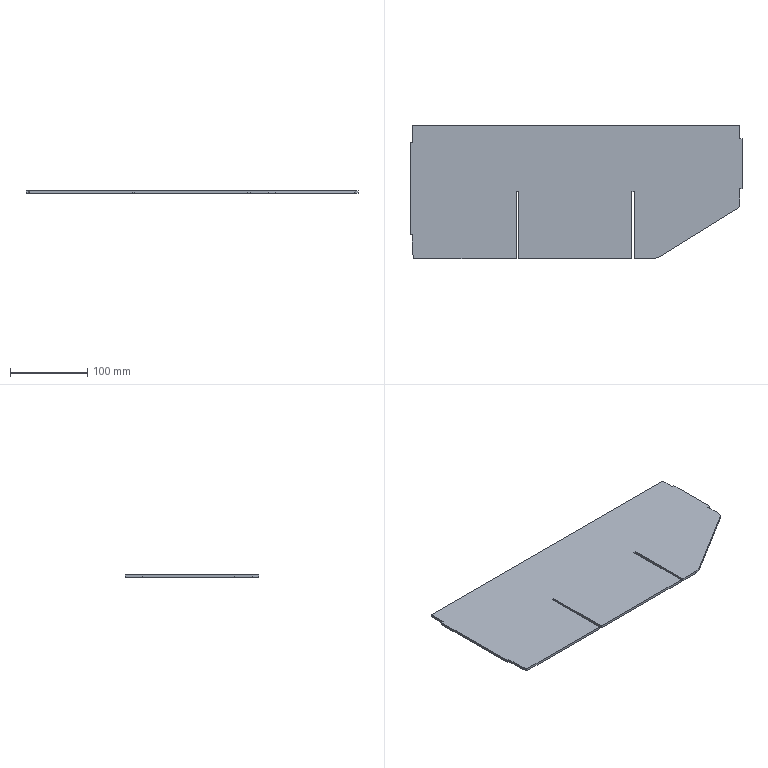Part | SolidWorks | features FlatPattern 1, SMBaseFlange 1, SheetMetal 1 | 1 solid | 26 faces | box 431 x 173.7 x 3.2 mm | volume 224566 mm3 | plane 26
STEP:
#1=CARTESIAN_POINT('',(206.522,-13.627,0.));
#2=VERTEX_POINT('',#1);
#3=CARTESIAN_POINT('',(-218.478,-13.627,0.));
#4=VERTEX_POINT('',#3);
#5=CARTESIAN_POINT('',(-218.478,-13.627,0.));
#6=DIRECTION('',(-1.,0.,0.));
#7=VECTOR('',#6,1000.);
#8=LINE('',#5,#7);
#9=EDGE_CURVE('',#2,#4,#8,.T.);
#10=ORIENTED_EDGE('',*,*,#9,.T.);
#11=CARTESIAN_POINT('',(-218.478,-13.627,3.2));
#12=VERTEX_POINT('',#11);
#13=CARTESIAN_POINT('',(-218.478,-13.627,3.2));
#14=DIRECTION('',(0.,0.,-1.));
#15=VECTOR('',#14,1000.);
#16=LINE('',#13,#15);
#17=EDGE_CURVE('',#12,#4,#16,.T.);
#18=ORIENTED_EDGE('',*,*,#17,.F.);
#19=CARTESIAN_POINT('',(206.522,-13.627,3.2));
#20=VERTEX_POINT('',#19);
#21=CARTESIAN_POINT('',(-218.478,-13.627,3.2));
#22=DIRECTION('',(-1.,0.,0.));
#23=VECTOR('',#22,1000.);
#24=LINE('',#21,#23);
#25=EDGE_CURVE('',#20,#12,#24,.T.);
#26=ORIENTED_EDGE('',*,*,#25,.F.);
#27=CARTESIAN_POINT('',(206.522,-13.627,3.2));
#28=DIRECTION('',(0.,0.,-1.));
#29=VECTOR('',#28,1000.);
#30=LINE('',#27,#29);
#31=EDGE_CURVE('',#20,#2,#30,.T.);
#32=ORIENTED_EDGE('',*,*,#31,.T.);
#33=EDGE_LOOP('',(#10,#18,#26,#32));
#34=FACE_OUTER_BOUND('',#33,.T.);
#35=CARTESIAN_POINT('',(-218.478,-13.627,3.2));
#36=DIRECTION('',(0.,-1.,0.));
#37=DIRECTION('',(0.,0.,-1.));
#38=AXIS2_PLACEMENT_3D('',#35,#36,#37);
#39=PLANE('',#38);
#40=ADVANCED_FACE('',(#34),#39,.F.);
#41=CARTESIAN_POINT('',(-218.478,-36.127,0.));
#42=VERTEX_POINT('',#41);
#43=CARTESIAN_POINT('',(-218.478,-13.627,0.));
#44=DIRECTION('',(0.,-1.,0.));
#45=VECTOR('',#44,1000.);
#46=LINE('',#43,#45);
#47=EDGE_CURVE('',#4,#42,#46,.T.);
#48=ORIENTED_EDGE('',*,*,#47,.T.);
#49=CARTESIAN_POINT('',(-218.478,-36.127,3.2));
#50=VERTEX_POINT('',#49);
#51=CARTESIAN_POINT('',(-218.478,-36.127,3.2));
#52=DIRECTION('',(0.,0.,-1.));
#53=VECTOR('',#52,1000.);
#54=LINE('',#51,#53);
#55=EDGE_CURVE('',#50,#42,#54,.T.);
#56=ORIENTED_EDGE('',*,*,#55,.F.);
#57=CARTESIAN_POINT('',(-218.478,-13.627,3.2));
#58=DIRECTION('',(0.,-1.,0.));
#59=VECTOR('',#58,1000.);
#60=LINE('',#57,#59);
#61=EDGE_CURVE('',#12,#50,#60,.T.);
#62=ORIENTED_EDGE('',*,*,#61,.F.);
#63=ORIENTED_EDGE('',*,*,#17,.T.);
#64=EDGE_LOOP('',(#48,#56,#62,#63));
#65=FACE_OUTER_BOUND('',#64,.T.);
#66=CARTESIAN_POINT('',(-218.478,-13.627,3.2));
#67=DIRECTION('',(1.,0.,0.));
#68=DIRECTION('',(0.,1.,0.));
#69=AXIS2_PLACEMENT_3D('',#66,#67,#68);
#70=PLANE('',#69);
#71=ADVANCED_FACE('',(#65),#70,.F.);
#72=CARTESIAN_POINT('',(-221.478,-36.127,0.));
#73=VERTEX_POINT('',#72);
#74=CARTESIAN_POINT('',(-221.478,-36.127,0.));
#75=DIRECTION('',(-1.,0.,0.));
#76=VECTOR('',#75,1000.);
#77=LINE('',#74,#76);
#78=EDGE_CURVE('',#42,#73,#77,.T.);
#79=ORIENTED_EDGE('',*,*,#78,.T.);
#80=CARTESIAN_POINT('',(-221.478,-36.127,3.2));
#81=VERTEX_POINT('',#80);
#82=CARTESIAN_POINT('',(-221.478,-36.127,3.2));
#83=DIRECTION('',(0.,0.,-1.));
#84=VECTOR('',#83,1000.);
#85=LINE('',#82,#84);
#86=EDGE_CURVE('',#81,#73,#85,.T.);
#87=ORIENTED_EDGE('',*,*,#86,.F.);
#88=CARTESIAN_POINT('',(-221.478,-36.127,3.2));
#89=DIRECTION('',(-1.,0.,0.));
#90=VECTOR('',#89,1000.);
#91=LINE('',#88,#90);
#92=EDGE_CURVE('',#50,#81,#91,.T.);
#93=ORIENTED_EDGE('',*,*,#92,.F.);
#94=ORIENTED_EDGE('',*,*,#55,.T.);
#95=EDGE_LOOP('',(#79,#87,#93,#94));
#96=FACE_OUTER_BOUND('',#95,.T.);
#97=CARTESIAN_POINT('',(-221.478,-36.127,3.2));
#98=DIRECTION('',(0.,-1.,0.));
#99=DIRECTION('',(0.,0.,-1.));
#100=AXIS2_PLACEMENT_3D('',#97,#98,#99);
#101=PLANE('',#100);
#102=ADVANCED_FACE('',(#96),#101,.F.);
#103=CARTESIAN_POINT('',(-221.478,-156.127,0.));
#104=VERTEX_POINT('',#103);
#105=CARTESIAN_POINT('',(-221.478,-156.127,0.));
#106=DIRECTION('',(0.,-1.,0.));
#107=VECTOR('',#106,1000.);
#108=LINE('',#105,#107);
#109=EDGE_CURVE('',#73,#104,#108,.T.);
#110=ORIENTED_EDGE('',*,*,#109,.T.);
#111=CARTESIAN_POINT('',(-221.478,-156.127,3.2));
#112=VERTEX_POINT('',#111);
#113=CARTESIAN_POINT('',(-221.478,-156.127,3.2));
#114=DIRECTION('',(0.,0.,-1.));
#115=VECTOR('',#114,1000.);
#116=LINE('',#113,#115);
#117=EDGE_CURVE('',#112,#104,#116,.T.);
#118=ORIENTED_EDGE('',*,*,#117,.F.);
#119=CARTESIAN_POINT('',(-221.478,-156.127,3.2));
#120=DIRECTION('',(0.,-1.,0.));
#121=VECTOR('',#120,1000.);
#122=LINE('',#119,#121);
#123=EDGE_CURVE('',#81,#112,#122,.T.);
#124=ORIENTED_EDGE('',*,*,#123,.F.);
#125=ORIENTED_EDGE('',*,*,#86,.T.);
#126=EDGE_LOOP('',(#110,#118,#124,#125));
#127=FACE_OUTER_BOUND('',#126,.T.);
#128=CARTESIAN_POINT('',(-221.478,-156.127,3.2));
#129=DIRECTION('',(1.,0.,0.));
#130=DIRECTION('',(0.,0.,-1.));
#131=AXIS2_PLACEMENT_3D('',#128,#129,#130);
#132=PLANE('',#131);
#133=ADVANCED_FACE('',(#127),#132,.F.);
#134=CARTESIAN_POINT('',(-218.478,-156.127,0.));
#135=VERTEX_POINT('',#134);
#136=CARTESIAN_POINT('',(-218.478,-156.127,0.));
#137=DIRECTION('',(1.,0.,0.));
#138=VECTOR('',#137,1000.);
#139=LINE('',#136,#138);
#140=EDGE_CURVE('',#104,#135,#139,.T.);
#141=ORIENTED_EDGE('',*,*,#140,.T.);
#142=CARTESIAN_POINT('',(-218.478,-156.127,3.2));
#143=VERTEX_POINT('',#142);
#144=CARTESIAN_POINT('',(-218.478,-156.127,3.2));
#145=DIRECTION('',(0.,0.,-1.));
#146=VECTOR('',#145,1000.);
#147=LINE('',#144,#146);
#148=EDGE_CURVE('',#143,#135,#147,.T.);
#149=ORIENTED_EDGE('',*,*,#148,.F.);
#150=CARTESIAN_POINT('',(-218.478,-156.127,3.2));
#151=DIRECTION('',(1.,0.,0.));
#152=VECTOR('',#151,1000.);
#153=LINE('',#150,#152);
#154=EDGE_CURVE('',#112,#143,#153,.T.);
#155=ORIENTED_EDGE('',*,*,#154,.F.);
#156=ORIENTED_EDGE('',*,*,#117,.T.);
#157=EDGE_LOOP('',(#141,#149,#155,#156));
#158=FACE_OUTER_BOUND('',#157,.T.);
#159=CARTESIAN_POINT('',(-218.478,-156.127,3.2));
#160=DIRECTION('',(0.,1.,0.));
#161=DIRECTION('',(0.,0.,1.));
#162=AXIS2_PLACEMENT_3D('',#159,#160,#161);
#163=PLANE('',#162);
#164=ADVANCED_FACE('',(#158),#163,.F.);
#165=CARTESIAN_POINT('',(-218.478,-178.627,0.));
#166=VERTEX_POINT('',#165);
#167=CARTESIAN_POINT('',(-218.478,-156.127,0.));
#168=DIRECTION('',(0.,-1.,0.));
#169=VECTOR('',#168,1000.);
#170=LINE('',#167,#169);
#171=EDGE_CURVE('',#135,#166,#170,.T.);
#172=ORIENTED_EDGE('',*,*,#171,.T.);
#173=CARTESIAN_POINT('',(-218.478,-178.627,3.2));
#174=VERTEX_POINT('',#173);
#175=CARTESIAN_POINT('',(-218.478,-178.627,3.2));
#176=DIRECTION('',(0.,0.,-1.));
#177=VECTOR('',#176,1000.);
#178=LINE('',#175,#177);
#179=EDGE_CURVE('',#174,#166,#178,.T.);
#180=ORIENTED_EDGE('',*,*,#179,.F.);
#181=CARTESIAN_POINT('',(-218.478,-156.127,3.2));
#182=DIRECTION('',(0.,-1.,0.));
#183=VECTOR('',#182,1000.);
#184=LINE('',#181,#183);
#185=EDGE_CURVE('',#143,#174,#184,.T.);
#186=ORIENTED_EDGE('',*,*,#185,.F.);
#187=ORIENTED_EDGE('',*,*,#148,.T.);
#188=EDGE_LOOP('',(#172,#180,#186,#187));
#189=FACE_OUTER_BOUND('',#188,.T.);
#190=CARTESIAN_POINT('',(-218.478,-156.127,3.2));
#191=DIRECTION('',(1.,0.,0.));
#192=DIRECTION('',(0.,0.,-1.));
#193=AXIS2_PLACEMENT_3D('',#190,#191,#192);
#194=PLANE('',#193);
#195=ADVANCED_FACE('',(#189),#194,.F.);
#196=CARTESIAN_POINT('',(-216.628,-187.327,0.));
#197=VERTEX_POINT('',#196);
#198=CARTESIAN_POINT('',(-218.478,-178.627,0.));
#199=DIRECTION('',(0.208,-0.9781,0.));
#200=VECTOR('',#199,1000.);
#201=LINE('',#198,#200);
#202=EDGE_CURVE('',#166,#197,#201,.T.);
#203=ORIENTED_EDGE('',*,*,#202,.T.);
#204=CARTESIAN_POINT('',(-216.628,-187.327,3.2));
#205=VERTEX_POINT('',#204);
#206=CARTESIAN_POINT('',(-216.628,-187.327,3.2));
#207=DIRECTION('',(0.,0.,-1.));
#208=VECTOR('',#207,1000.);
#209=LINE('',#206,#208);
#210=EDGE_CURVE('',#205,#197,#209,.T.);
#211=ORIENTED_EDGE('',*,*,#210,.F.);
#212=CARTESIAN_POINT('',(-218.478,-178.627,3.2));
#213=DIRECTION('',(0.208,-0.9781,0.));
#214=VECTOR('',#213,1000.);
#215=LINE('',#212,#214);
#216=EDGE_CURVE('',#174,#205,#215,.T.);
#217=ORIENTED_EDGE('',*,*,#216,.F.);
#218=ORIENTED_EDGE('',*,*,#179,.T.);
#219=EDGE_LOOP('',(#203,#211,#217,#218));
#220=FACE_OUTER_BOUND('',#219,.T.);
#221=CARTESIAN_POINT('',(-218.478,-178.627,3.2));
#222=DIRECTION('',(0.9781,0.208,0.));
#223=DIRECTION('',(-0.208,0.9781,0.));
#224=AXIS2_PLACEMENT_3D('',#221,#222,#223);
#225=PLANE('',#224);
#226=ADVANCED_FACE('',(#220),#225,.F.);
#227=CARTESIAN_POINT('',(-83.478,-187.327,0.));
#228=VERTEX_POINT('',#227);
#229=CARTESIAN_POINT('',(-216.628,-187.327,0.));
#230=DIRECTION('',(1.,0.,0.));
#231=VECTOR('',#230,1000.);
#232=LINE('',#229,#231);
#233=EDGE_CURVE('',#197,#228,#232,.T.);
#234=ORIENTED_EDGE('',*,*,#233,.T.);
#235=CARTESIAN_POINT('',(-83.478,-187.327,3.2));
#236=VERTEX_POINT('',#235);
#237=CARTESIAN_POINT('',(-83.478,-187.327,3.2));
#238=DIRECTION('',(0.,0.,-1.));
#239=VECTOR('',#238,1000.);
#240=LINE('',#237,#239);
#241=EDGE_CURVE('',#236,#228,#240,.T.);
#242=ORIENTED_EDGE('',*,*,#241,.F.);
#243=CARTESIAN_POINT('',(-216.628,-187.327,3.2));
#244=DIRECTION('',(1.,0.,0.));
#245=VECTOR('',#244,1000.);
#246=LINE('',#243,#245);
#247=EDGE_CURVE('',#205,#236,#246,.T.);
#248=ORIENTED_EDGE('',*,*,#247,.F.);
#249=ORIENTED_EDGE('',*,*,#210,.T.);
#250=EDGE_LOOP('',(#234,#242,#248,#249));
#251=FACE_OUTER_BOUND('',#250,.T.);
#252=CARTESIAN_POINT('',(-216.628,-187.327,3.2));
#253=DIRECTION('',(0.,1.,0.));
#254=DIRECTION('',(-1.,0.,0.));
#255=AXIS2_PLACEMENT_3D('',#252,#253,#254);
#256=PLANE('',#255);
#257=ADVANCED_FACE('',(#251),#256,.F.);
#258=CARTESIAN_POINT('',(-83.478,-100.327,0.));
#259=VERTEX_POINT('',#258);
#260=CARTESIAN_POINT('',(-83.478,-187.327,0.));
#261=DIRECTION('',(0.,1.,0.));
#262=VECTOR('',#261,1000.);
#263=LINE('',#260,#262);
#264=EDGE_CURVE('',#228,#259,#263,.T.);
#265=ORIENTED_EDGE('',*,*,#264,.T.);
#266=CARTESIAN_POINT('',(-83.478,-100.327,3.2));
#267=VERTEX_POINT('',#266);
#268=CARTESIAN_POINT('',(-83.478,-100.327,3.2));
#269=DIRECTION('',(0.,0.,-1.));
#270=VECTOR('',#269,1000.);
#271=LINE('',#268,#270);
#272=EDGE_CURVE('',#267,#259,#271,.T.);
#273=ORIENTED_EDGE('',*,*,#272,.F.);
#274=CARTESIAN_POINT('',(-83.478,-187.327,3.2));
#275=DIRECTION('',(0.,1.,0.));
#276=VECTOR('',#275,1000.);
#277=LINE('',#274,#276);
#278=EDGE_CURVE('',#236,#267,#277,.T.);
#279=ORIENTED_EDGE('',*,*,#278,.F.);
#280=ORIENTED_EDGE('',*,*,#241,.T.);
#281=EDGE_LOOP('',(#265,#273,#279,#280));
#282=FACE_OUTER_BOUND('',#281,.T.);
#283=CARTESIAN_POINT('',(-83.478,-187.327,3.2));
#284=DIRECTION('',(-1.,0.,0.));
#285=DIRECTION('',(0.,0.,1.));
#286=AXIS2_PLACEMENT_3D('',#283,#284,#285);
#287=PLANE('',#286);
#288=ADVANCED_FACE('',(#282),#287,.F.);
#289=CARTESIAN_POINT('',(-80.278,-100.327,0.));
#290=VERTEX_POINT('',#289);
#291=CARTESIAN_POINT('',(-83.478,-100.327,0.));
#292=DIRECTION('',(1.,0.,0.));
#293=VECTOR('',#292,1000.);
#294=LINE('',#291,#293);
#295=EDGE_CURVE('',#259,#290,#294,.T.);
#296=ORIENTED_EDGE('',*,*,#295,.T.);
#297=CARTESIAN_POINT('',(-80.278,-100.327,3.2));
#298=VERTEX_POINT('',#297);
#299=CARTESIAN_POINT('',(-80.278,-100.327,3.2));
#300=DIRECTION('',(0.,0.,-1.));
#301=VECTOR('',#300,1000.);
#302=LINE('',#299,#301);
#303=EDGE_CURVE('',#298,#290,#302,.T.);
#304=ORIENTED_EDGE('',*,*,#303,.F.);
#305=CARTESIAN_POINT('',(-83.478,-100.327,3.2));
#306=DIRECTION('',(1.,0.,0.));
#307=VECTOR('',#306,1000.);
#308=LINE('',#305,#307);
#309=EDGE_CURVE('',#267,#298,#308,.T.);
#310=ORIENTED_EDGE('',*,*,#309,.F.);
#311=ORIENTED_EDGE('',*,*,#272,.T.);
#312=EDGE_LOOP('',(#296,#304,#310,#311));
#313=FACE_OUTER_BOUND('',#312,.T.);
#314=CARTESIAN_POINT('',(-83.478,-100.327,3.2));
#315=DIRECTION('',(0.,1.,0.));
#316=DIRECTION('',(0.,0.,1.));
#317=AXIS2_PLACEMENT_3D('',#314,#315,#316);
#318=PLANE('',#317);
#319=ADVANCED_FACE('',(#313),#318,.F.);
#320=CARTESIAN_POINT('',(-80.278,-187.327,0.));
#321=VERTEX_POINT('',#320);
#322=CARTESIAN_POINT('',(-80.278,-100.327,0.));
#323=DIRECTION('',(0.,-1.,0.));
#324=VECTOR('',#323,1000.);
#325=LINE('',#322,#324);
#326=EDGE_CURVE('',#290,#321,#325,.T.);
#327=ORIENTED_EDGE('',*,*,#326,.T.);
#328=CARTESIAN_POINT('',(-80.278,-187.327,3.2));
#329=VERTEX_POINT('',#328);
#330=CARTESIAN_POINT('',(-80.278,-187.327,3.2));
#331=DIRECTION('',(0.,0.,-1.));
#332=VECTOR('',#331,1000.);
#333=LINE('',#330,#332);
#334=EDGE_CURVE('',#329,#321,#333,.T.);
#335=ORIENTED_EDGE('',*,*,#334,.F.);
#336=CARTESIAN_POINT('',(-80.278,-100.327,3.2));
#337=DIRECTION('',(0.,-1.,0.));
#338=VECTOR('',#337,1000.);
#339=LINE('',#336,#338);
#340=EDGE_CURVE('',#298,#329,#339,.T.);
#341=ORIENTED_EDGE('',*,*,#340,.F.);
#342=ORIENTED_EDGE('',*,*,#303,.T.);
#343=EDGE_LOOP('',(#327,#335,#341,#342));
#344=FACE_OUTER_BOUND('',#343,.T.);
#345=CARTESIAN_POINT('',(-80.278,-100.327,3.2));
#346=DIRECTION('',(1.,0.,0.));
#347=DIRECTION('',(0.,0.,-1.));
#348=AXIS2_PLACEMENT_3D('',#345,#346,#347);
#349=PLANE('',#348);
#350=ADVANCED_FACE('',(#344),#349,.F.);
#351=CARTESIAN_POINT('',(66.522,-187.327,0.));
#352=VERTEX_POINT('',#351);
#353=CARTESIAN_POINT('',(-80.278,-187.327,0.));
#354=DIRECTION('',(1.,0.,0.));
#355=VECTOR('',#354,1000.);
#356=LINE('',#353,#355);
#357=EDGE_CURVE('',#321,#352,#356,.T.);
#358=ORIENTED_EDGE('',*,*,#357,.T.);
#359=CARTESIAN_POINT('',(66.522,-187.327,3.2));
#360=VERTEX_POINT('',#359);
#361=CARTESIAN_POINT('',(66.522,-187.327,3.2));
#362=DIRECTION('',(0.,0.,-1.));
#363=VECTOR('',#362,1000.);
#364=LINE('',#361,#363);
#365=EDGE_CURVE('',#360,#352,#364,.T.);
#366=ORIENTED_EDGE('',*,*,#365,.F.);
#367=CARTESIAN_POINT('',(-80.278,-187.327,3.2));
#368=DIRECTION('',(1.,0.,0.));
#369=VECTOR('',#368,1000.);
#370=LINE('',#367,#369);
#371=EDGE_CURVE('',#329,#360,#370,.T.);
#372=ORIENTED_EDGE('',*,*,#371,.F.);
#373=ORIENTED_EDGE('',*,*,#334,.T.);
#374=EDGE_LOOP('',(#358,#366,#372,#373));
#375=FACE_OUTER_BOUND('',#374,.T.);
#376=CARTESIAN_POINT('',(-80.278,-187.327,3.2));
#377=DIRECTION('',(0.,1.,0.));
#378=DIRECTION('',(0.,0.,1.));
#379=AXIS2_PLACEMENT_3D('',#376,#377,#378);
#380=PLANE('',#379);
#381=ADVANCED_FACE('',(#375),#380,.F.);
#382=CARTESIAN_POINT('',(66.522,-100.327,0.));
#383=VERTEX_POINT('',#382);
#384=CARTESIAN_POINT('',(66.522,-187.327,0.));
#385=DIRECTION('',(0.,1.,0.));
#386=VECTOR('',#385,1000.);
#387=LINE('',#384,#386);
#388=EDGE_CURVE('',#352,#383,#387,.T.);
#389=ORIENTED_EDGE('',*,*,#388,.T.);
#390=CARTESIAN_POINT('',(66.522,-100.327,3.2));
#391=VERTEX_POINT('',#390);
#392=CARTESIAN_POINT('',(66.522,-100.327,3.2));
#393=DIRECTION('',(0.,0.,-1.));
#394=VECTOR('',#393,1000.);
#395=LINE('',#392,#394);
#396=EDGE_CURVE('',#391,#383,#395,.T.);
#397=ORIENTED_EDGE('',*,*,#396,.F.);
#398=CARTESIAN_POINT('',(66.522,-187.327,3.2));
#399=DIRECTION('',(0.,1.,0.));
#400=VECTOR('',#399,1000.);
#401=LINE('',#398,#400);
#402=EDGE_CURVE('',#360,#391,#401,.T.);
#403=ORIENTED_EDGE('',*,*,#402,.F.);
#404=ORIENTED_EDGE('',*,*,#365,.T.);
#405=EDGE_LOOP('',(#389,#397,#403,#404));
#406=FACE_OUTER_BOUND('',#405,.T.);
#407=CARTESIAN_POINT('',(66.522,-187.327,3.2));
#408=DIRECTION('',(-1.,0.,0.));
#409=DIRECTION('',(0.,0.,1.));
#410=AXIS2_PLACEMENT_3D('',#407,#408,#409);
#411=PLANE('',#410);
#412=ADVANCED_FACE('',(#406),#411,.F.);
#413=CARTESIAN_POINT('',(69.722,-100.327,0.));
#414=VERTEX_POINT('',#413);
#415=CARTESIAN_POINT('',(66.522,-100.327,0.));
#416=DIRECTION('',(1.,0.,0.));
#417=VECTOR('',#416,1000.);
#418=LINE('',#415,#417);
#419=EDGE_CURVE('',#383,#414,#418,.T.);
#420=ORIENTED_EDGE('',*,*,#419,.T.);
#421=CARTESIAN_POINT('',(69.722,-100.327,3.2));
#422=VERTEX_POINT('',#421);
#423=CARTESIAN_POINT('',(69.722,-100.327,3.2));
#424=DIRECTION('',(0.,0.,-1.));
#425=VECTOR('',#424,1000.);
#426=LINE('',#423,#425);
#427=EDGE_CURVE('',#422,#414,#426,.T.);
#428=ORIENTED_EDGE('',*,*,#427,.F.);
#429=CARTESIAN_POINT('',(66.522,-100.327,3.2));
#430=DIRECTION('',(1.,0.,0.));
#431=VECTOR('',#430,1000.);
#432=LINE('',#429,#431);
#433=EDGE_CURVE('',#391,#422,#432,.T.);
#434=ORIENTED_EDGE('',*,*,#433,.F.);
#435=ORIENTED_EDGE('',*,*,#396,.T.);
#436=EDGE_LOOP('',(#420,#428,#434,#435));
#437=FACE_OUTER_BOUND('',#436,.T.);
#438=CARTESIAN_POINT('',(66.522,-100.327,3.2));
#439=DIRECTION('',(0.,1.,0.));
#440=DIRECTION('',(0.,0.,1.));
#441=AXIS2_PLACEMENT_3D('',#438,#439,#440);
#442=PLANE('',#441);
#443=ADVANCED_FACE('',(#437),#442,.F.);
#444=CARTESIAN_POINT('',(69.722,-187.327,0.));
#445=VERTEX_POINT('',#444);
#446=CARTESIAN_POINT('',(69.722,-100.327,0.));
#447=DIRECTION('',(0.,-1.,0.));
#448=VECTOR('',#447,1000.);
#449=LINE('',#446,#448);
#450=EDGE_CURVE('',#414,#445,#449,.T.);
#451=ORIENTED_EDGE('',*,*,#450,.T.);
#452=CARTESIAN_POINT('',(69.722,-187.327,3.2));
#453=VERTEX_POINT('',#452);
#454=CARTESIAN_POINT('',(69.722,-187.327,3.2));
#455=DIRECTION('',(0.,0.,-1.));
#456=VECTOR('',#455,1000.);
#457=LINE('',#454,#456);
#458=EDGE_CURVE('',#453,#445,#457,.T.);
#459=ORIENTED_EDGE('',*,*,#458,.F.);
#460=CARTESIAN_POINT('',(69.722,-100.327,3.2));
#461=DIRECTION('',(0.,-1.,0.));
#462=VECTOR('',#461,1000.);
#463=LINE('',#460,#462);
#464=EDGE_CURVE('',#422,#453,#463,.T.);
#465=ORIENTED_EDGE('',*,*,#464,.F.);
#466=ORIENTED_EDGE('',*,*,#427,.T.);
#467=EDGE_LOOP('',(#451,#459,#465,#466));
#468=FACE_OUTER_BOUND('',#467,.T.);
#469=CARTESIAN_POINT('',(69.722,-100.327,3.2));
#470=DIRECTION('',(1.,0.,0.));
#471=DIRECTION('',(0.,0.,-1.));
#472=AXIS2_PLACEMENT_3D('',#469,#470,#471);
#473=PLANE('',#472);
#474=ADVANCED_FACE('',(#468),#473,.F.);
#475=CARTESIAN_POINT('',(93.322,-187.327,0.));
#476=VERTEX_POINT('',#475);
#477=CARTESIAN_POINT('',(69.722,-187.327,0.));
#478=DIRECTION('',(1.,0.,0.));
#479=VECTOR('',#478,1000.);
#480=LINE('',#477,#479);
#481=EDGE_CURVE('',#445,#476,#480,.T.);
#482=ORIENTED_EDGE('',*,*,#481,.T.);
#483=CARTESIAN_POINT('',(93.322,-187.327,3.2));
#484=VERTEX_POINT('',#483);
#485=CARTESIAN_POINT('',(93.322,-187.327,3.2));
#486=DIRECTION('',(0.,0.,-1.));
#487=VECTOR('',#486,1000.);
#488=LINE('',#485,#487);
#489=EDGE_CURVE('',#484,#476,#488,.T.);
#490=ORIENTED_EDGE('',*,*,#489,.F.);
#491=CARTESIAN_POINT('',(69.722,-187.327,3.2));
#492=DIRECTION('',(1.,0.,0.));
#493=VECTOR('',#492,1000.);
#494=LINE('',#491,#493);
#495=EDGE_CURVE('',#453,#484,#494,.T.);
#496=ORIENTED_EDGE('',*,*,#495,.F.);
#497=ORIENTED_EDGE('',*,*,#458,.T.);
#498=EDGE_LOOP('',(#482,#490,#496,#497));
#499=FACE_OUTER_BOUND('',#498,.T.);
#500=CARTESIAN_POINT('',(69.722,-187.327,3.2));
#501=DIRECTION('',(0.,1.,0.));
#502=DIRECTION('',(-1.,0.,0.));
#503=AXIS2_PLACEMENT_3D('',#500,#501,#502);
#504=PLANE('',#503);
#505=ADVANCED_FACE('',(#499),#504,.F.);
#506=CARTESIAN_POINT('',(102.573,-184.694,0.));
#507=VERTEX_POINT('',#506);
#508=CARTESIAN_POINT('',(93.322,-187.327,0.));
#509=DIRECTION('',(0.9618,0.2737,0.));
#510=VECTOR('',#509,1000.);
#511=LINE('',#508,#510);
#512=EDGE_CURVE('',#476,#507,#511,.T.);
#513=ORIENTED_EDGE('',*,*,#512,.T.);
#514=CARTESIAN_POINT('',(102.573,-184.694,3.2));
#515=VERTEX_POINT('',#514);
#516=CARTESIAN_POINT('',(102.573,-184.694,3.2));
#517=DIRECTION('',(0.,0.,-1.));
#518=VECTOR('',#517,1000.);
#519=LINE('',#516,#518);
#520=EDGE_CURVE('',#515,#507,#519,.T.);
#521=ORIENTED_EDGE('',*,*,#520,.F.);
#522=CARTESIAN_POINT('',(93.322,-187.327,3.2));
#523=DIRECTION('',(0.9618,0.2737,0.));
#524=VECTOR('',#523,1000.);
#525=LINE('',#522,#524);
#526=EDGE_CURVE('',#484,#515,#525,.T.);
#527=ORIENTED_EDGE('',*,*,#526,.F.);
#528=ORIENTED_EDGE('',*,*,#489,.T.);
#529=EDGE_LOOP('',(#513,#521,#527,#528));
#530=FACE_OUTER_BOUND('',#529,.T.);
#531=CARTESIAN_POINT('',(93.322,-187.327,3.2));
#532=DIRECTION('',(-0.2737,0.9618,0.));
#533=DIRECTION('',(-0.9618,-0.2737,0.));
#534=AXIS2_PLACEMENT_3D('',#531,#532,#533);
#535=PLANE('',#534);
#536=ADVANCED_FACE('',(#530),#535,.F.);
#537=CARTESIAN_POINT('',(205.471,-120.96,0.));
#538=VERTEX_POINT('',#537);
#539=CARTESIAN_POINT('',(102.573,-184.694,0.));
#540=DIRECTION('',(0.8501,0.5266,0.));
#541=VECTOR('',#540,1000.);
#542=LINE('',#539,#541);
#543=EDGE_CURVE('',#507,#538,#542,.T.);
#544=ORIENTED_EDGE('',*,*,#543,.T.);
#545=CARTESIAN_POINT('',(205.471,-120.96,3.2));
#546=VERTEX_POINT('',#545);
#547=CARTESIAN_POINT('',(205.471,-120.96,3.2));
#548=DIRECTION('',(0.,0.,-1.));
#549=VECTOR('',#548,1000.);
#550=LINE('',#547,#549);
#551=EDGE_CURVE('',#546,#538,#550,.T.);
#552=ORIENTED_EDGE('',*,*,#551,.F.);
#553=CARTESIAN_POINT('',(102.573,-184.694,3.2));
#554=DIRECTION('',(0.8501,0.5266,0.));
#555=VECTOR('',#554,1000.);
#556=LINE('',#553,#555);
#557=EDGE_CURVE('',#515,#546,#556,.T.);
#558=ORIENTED_EDGE('',*,*,#557,.F.);
#559=ORIENTED_EDGE('',*,*,#520,.T.);
#560=EDGE_LOOP('',(#544,#552,#558,#559));
#561=FACE_OUTER_BOUND('',#560,.T.);
#562=CARTESIAN_POINT('',(102.573,-184.694,3.2));
#563=DIRECTION('',(-0.5266,0.8501,0.));
#564=DIRECTION('',(-0.8501,-0.5266,0.));
#565=AXIS2_PLACEMENT_3D('',#562,#563,#564);
#566=PLANE('',#565);
#567=ADVANCED_FACE('',(#561),#566,.F.);
#568=CARTESIAN_POINT('',(206.522,-113.627,0.));
#569=VERTEX_POINT('',#568);
#570=CARTESIAN_POINT('',(206.522,-113.627,0.));
#571=DIRECTION('',(0.1418,0.9899,0.));
#572=VECTOR('',#571,1000.);
#573=LINE('',#570,#572);
#574=EDGE_CURVE('',#538,#569,#573,.T.);
#575=ORIENTED_EDGE('',*,*,#574,.T.);
#576=CARTESIAN_POINT('',(206.522,-113.627,3.2));
#577=VERTEX_POINT('',#576);
#578=CARTESIAN_POINT('',(206.522,-113.627,3.2));
#579=DIRECTION('',(0.,0.,-1.));
#580=VECTOR('',#579,1000.);
#581=LINE('',#578,#580);
#582=EDGE_CURVE('',#577,#569,#581,.T.);
#583=ORIENTED_EDGE('',*,*,#582,.F.);
#584=CARTESIAN_POINT('',(206.522,-113.627,3.2));
#585=DIRECTION('',(0.1418,0.9899,0.));
#586=VECTOR('',#585,1000.);
#587=LINE('',#584,#586);
#588=EDGE_CURVE('',#546,#577,#587,.T.);
#589=ORIENTED_EDGE('',*,*,#588,.F.);
#590=ORIENTED_EDGE('',*,*,#551,.T.);
#591=EDGE_LOOP('',(#575,#583,#589,#590));
#592=FACE_OUTER_BOUND('',#591,.T.);
#593=CARTESIAN_POINT('',(206.522,-113.627,3.2));
#594=DIRECTION('',(-0.9899,0.1418,0.));
#595=DIRECTION('',(-0.1418,-0.9899,0.));
#596=AXIS2_PLACEMENT_3D('',#593,#594,#595);
#597=PLANE('',#596);
#598=ADVANCED_FACE('',(#592),#597,.F.);
#599=CARTESIAN_POINT('',(206.522,-96.127,0.));
#600=VERTEX_POINT('',#599);
#601=CARTESIAN_POINT('',(206.522,-96.127,0.));
#602=DIRECTION('',(0.,1.,0.));
#603=VECTOR('',#602,1000.);
#604=LINE('',#601,#603);
#605=EDGE_CURVE('',#569,#600,#604,.T.);
#606=ORIENTED_EDGE('',*,*,#605,.T.);
#607=CARTESIAN_POINT('',(206.522,-96.127,3.2));
#608=VERTEX_POINT('',#607);
#609=CARTESIAN_POINT('',(206.522,-96.127,3.2));
#610=DIRECTION('',(0.,0.,-1.));
#611=VECTOR('',#610,1000.);
#612=LINE('',#609,#611);
#613=EDGE_CURVE('',#608,#600,#612,.T.);
#614=ORIENTED_EDGE('',*,*,#613,.F.);
#615=CARTESIAN_POINT('',(206.522,-96.127,3.2));
#616=DIRECTION('',(0.,1.,0.));
#617=VECTOR('',#616,1000.);
#618=LINE('',#615,#617);
#619=EDGE_CURVE('',#577,#608,#618,.T.);
#620=ORIENTED_EDGE('',*,*,#619,.F.);
#621=ORIENTED_EDGE('',*,*,#582,.T.);
#622=EDGE_LOOP('',(#606,#614,#620,#621));
#623=FACE_OUTER_BOUND('',#622,.T.);
#624=CARTESIAN_POINT('',(206.522,-96.127,3.2));
#625=DIRECTION('',(-1.,0.,0.));
#626=DIRECTION('',(0.,-1.,0.));
#627=AXIS2_PLACEMENT_3D('',#624,#625,#626);
#628=PLANE('',#627);
#629=ADVANCED_FACE('',(#623),#628,.F.);
#630=CARTESIAN_POINT('',(209.522,-96.127,0.));
#631=VERTEX_POINT('',#630);
#632=CARTESIAN_POINT('',(206.522,-96.127,0.));
#633=DIRECTION('',(1.,0.,0.));
#634=VECTOR('',#633,1000.);
#635=LINE('',#632,#634);
#636=EDGE_CURVE('',#600,#631,#635,.T.);
#637=ORIENTED_EDGE('',*,*,#636,.T.);
#638=CARTESIAN_POINT('',(209.522,-96.127,3.2));
#639=VERTEX_POINT('',#638);
#640=CARTESIAN_POINT('',(209.522,-96.127,3.2));
#641=DIRECTION('',(0.,0.,-1.));
#642=VECTOR('',#641,1000.);
#643=LINE('',#640,#642);
#644=EDGE_CURVE('',#639,#631,#643,.T.);
#645=ORIENTED_EDGE('',*,*,#644,.F.);
#646=CARTESIAN_POINT('',(206.522,-96.127,3.2));
#647=DIRECTION('',(1.,0.,0.));
#648=VECTOR('',#647,1000.);
#649=LINE('',#646,#648);
#650=EDGE_CURVE('',#608,#639,#649,.T.);
#651=ORIENTED_EDGE('',*,*,#650,.F.);
#652=ORIENTED_EDGE('',*,*,#613,.T.);
#653=EDGE_LOOP('',(#637,#645,#651,#652));
#654=FACE_OUTER_BOUND('',#653,.T.);
#655=CARTESIAN_POINT('',(206.522,-96.127,3.2));
#656=DIRECTION('',(0.,1.,0.));
#657=DIRECTION('',(0.,0.,1.));
#658=AXIS2_PLACEMENT_3D('',#655,#656,#657);
#659=PLANE('',#658);
#660=ADVANCED_FACE('',(#654),#659,.F.);
#661=CARTESIAN_POINT('',(209.522,-31.127,0.));
#662=VERTEX_POINT('',#661);
#663=CARTESIAN_POINT('',(209.522,-96.127,0.));
#664=DIRECTION('',(0.,1.,0.));
#665=VECTOR('',#664,1000.);
#666=LINE('',#663,#665);
#667=EDGE_CURVE('',#631,#662,#666,.T.);
#668=ORIENTED_EDGE('',*,*,#667,.T.);
#669=CARTESIAN_POINT('',(209.522,-31.127,3.2));
#670=VERTEX_POINT('',#669);
#671=CARTESIAN_POINT('',(209.522,-31.127,3.2));
#672=DIRECTION('',(0.,0.,-1.));
#673=VECTOR('',#672,1000.);
#674=LINE('',#671,#673);
#675=EDGE_CURVE('',#670,#662,#674,.T.);
#676=ORIENTED_EDGE('',*,*,#675,.F.);
#677=CARTESIAN_POINT('',(209.522,-96.127,3.2));
#678=DIRECTION('',(0.,1.,0.));
#679=VECTOR('',#678,1000.);
#680=LINE('',#677,#679);
#681=EDGE_CURVE('',#639,#670,#680,.T.);
#682=ORIENTED_EDGE('',*,*,#681,.F.);
#683=ORIENTED_EDGE('',*,*,#644,.T.);
#684=EDGE_LOOP('',(#668,#676,#682,#683));
#685=FACE_OUTER_BOUND('',#684,.T.);
#686=CARTESIAN_POINT('',(209.522,-96.127,3.2));
#687=DIRECTION('',(-1.,0.,0.));
#688=DIRECTION('',(0.,0.,1.));
#689=AXIS2_PLACEMENT_3D('',#686,#687,#688);
#690=PLANE('',#689);
#691=ADVANCED_FACE('',(#685),#690,.F.);
#692=CARTESIAN_POINT('',(206.522,-31.127,0.));
#693=VERTEX_POINT('',#692);
#694=CARTESIAN_POINT('',(209.522,-31.127,0.));
#695=DIRECTION('',(-1.,0.,0.));
#696=VECTOR('',#695,1000.);
#697=LINE('',#694,#696);
#698=EDGE_CURVE('',#662,#693,#697,.T.);
#699=ORIENTED_EDGE('',*,*,#698,.T.);
#700=CARTESIAN_POINT('',(206.522,-31.127,3.2));
#701=VERTEX_POINT('',#700);
#702=CARTESIAN_POINT('',(206.522,-31.127,3.2));
#703=DIRECTION('',(0.,0.,-1.));
#704=VECTOR('',#703,1000.);
#705=LINE('',#702,#704);
#706=EDGE_CURVE('',#701,#693,#705,.T.);
#707=ORIENTED_EDGE('',*,*,#706,.F.);
#708=CARTESIAN_POINT('',(209.522,-31.127,3.2));
#709=DIRECTION('',(-1.,0.,0.));
#710=VECTOR('',#709,1000.);
#711=LINE('',#708,#710);
#712=EDGE_CURVE('',#670,#701,#711,.T.);
#713=ORIENTED_EDGE('',*,*,#712,.F.);
#714=ORIENTED_EDGE('',*,*,#675,.T.);
#715=EDGE_LOOP('',(#699,#707,#713,#714));
#716=FACE_OUTER_BOUND('',#715,.T.);
#717=CARTESIAN_POINT('',(209.522,-31.127,3.2));
#718=DIRECTION('',(0.,-1.,0.));
#719=DIRECTION('',(0.,0.,-1.));
#720=AXIS2_PLACEMENT_3D('',#717,#718,#719);
#721=PLANE('',#720);
#722=ADVANCED_FACE('',(#716),#721,.F.);
#723=CARTESIAN_POINT('',(206.522,-13.627,0.));
#724=DIRECTION('',(0.,1.,0.));
#725=VECTOR('',#724,1000.);
#726=LINE('',#723,#725);
#727=EDGE_CURVE('',#693,#2,#726,.T.);
#728=ORIENTED_EDGE('',*,*,#727,.T.);
#729=ORIENTED_EDGE('',*,*,#31,.F.);
#730=CARTESIAN_POINT('',(206.522,-13.627,3.2));
#731=DIRECTION('',(0.,1.,0.));
#732=VECTOR('',#731,1000.);
#733=LINE('',#730,#732);
#734=EDGE_CURVE('',#701,#20,#733,.T.);
#735=ORIENTED_EDGE('',*,*,#734,.F.);
#736=ORIENTED_EDGE('',*,*,#706,.T.);
#737=EDGE_LOOP('',(#728,#729,#735,#736));
#738=FACE_OUTER_BOUND('',#737,.T.);
#739=CARTESIAN_POINT('',(206.522,-13.627,3.2));
#740=DIRECTION('',(-1.,0.,0.));
#741=DIRECTION('',(0.,-1.,0.));
#742=AXIS2_PLACEMENT_3D('',#739,#740,#741);
#743=PLANE('',#742);
#744=ADVANCED_FACE('',(#738),#743,.F.);
#745=ORIENTED_EDGE('',*,*,#25,.T.);
#746=ORIENTED_EDGE('',*,*,#61,.T.);
#747=ORIENTED_EDGE('',*,*,#92,.T.);
#748=ORIENTED_EDGE('',*,*,#123,.T.);
#749=ORIENTED_EDGE('',*,*,#154,.T.);
#750=ORIENTED_EDGE('',*,*,#185,.T.);
#751=ORIENTED_EDGE('',*,*,#216,.T.);
#752=ORIENTED_EDGE('',*,*,#247,.T.);
#753=ORIENTED_EDGE('',*,*,#278,.T.);
#754=ORIENTED_EDGE('',*,*,#309,.T.);
#755=ORIENTED_EDGE('',*,*,#340,.T.);
#756=ORIENTED_EDGE('',*,*,#371,.T.);
#757=ORIENTED_EDGE('',*,*,#402,.T.);
#758=ORIENTED_EDGE('',*,*,#433,.T.);
#759=ORIENTED_EDGE('',*,*,#464,.T.);
#760=ORIENTED_EDGE('',*,*,#495,.T.);
#761=ORIENTED_EDGE('',*,*,#526,.T.);
#762=ORIENTED_EDGE('',*,*,#557,.T.);
#763=ORIENTED_EDGE('',*,*,#588,.T.);
#764=ORIENTED_EDGE('',*,*,#619,.T.);
#765=ORIENTED_EDGE('',*,*,#650,.T.);
#766=ORIENTED_EDGE('',*,*,#681,.T.);
#767=ORIENTED_EDGE('',*,*,#712,.T.);
#768=ORIENTED_EDGE('',*,*,#734,.T.);
#769=EDGE_LOOP('',(#745,#746,#747,#748,#749,#750,#751,#752,#753,#754,#755,#756,#757,#758,#759,#760,#761,#762,#763,#764,#765,#766,#767,#768));
#770=FACE_OUTER_BOUND('',#769,.T.);
#771=CARTESIAN_POINT('',(0.,0.,3.2));
#772=DIRECTION('',(0.,0.,-1.));
#773=DIRECTION('',(-1.,0.,0.));
#774=AXIS2_PLACEMENT_3D('',#771,#772,#773);
#775=PLANE('',#774);
#776=ADVANCED_FACE('',(#770),#775,.F.);
#777=ORIENTED_EDGE('',*,*,#9,.F.);
#778=ORIENTED_EDGE('',*,*,#727,.F.);
#779=ORIENTED_EDGE('',*,*,#698,.F.);
#780=ORIENTED_EDGE('',*,*,#667,.F.);
#781=ORIENTED_EDGE('',*,*,#636,.F.);
#782=ORIENTED_EDGE('',*,*,#605,.F.);
#783=ORIENTED_EDGE('',*,*,#574,.F.);
#784=ORIENTED_EDGE('',*,*,#543,.F.);
#785=ORIENTED_EDGE('',*,*,#512,.F.);
#786=ORIENTED_EDGE('',*,*,#481,.F.);
#787=ORIENTED_EDGE('',*,*,#450,.F.);
#788=ORIENTED_EDGE('',*,*,#419,.F.);
#789=ORIENTED_EDGE('',*,*,#388,.F.);
#790=ORIENTED_EDGE('',*,*,#357,.F.);
#791=ORIENTED_EDGE('',*,*,#326,.F.);
#792=ORIENTED_EDGE('',*,*,#295,.F.);
#793=ORIENTED_EDGE('',*,*,#264,.F.);
#794=ORIENTED_EDGE('',*,*,#233,.F.);
#795=ORIENTED_EDGE('',*,*,#202,.F.);
#796=ORIENTED_EDGE('',*,*,#171,.F.);
#797=ORIENTED_EDGE('',*,*,#140,.F.);
#798=ORIENTED_EDGE('',*,*,#109,.F.);
#799=ORIENTED_EDGE('',*,*,#78,.F.);
#800=ORIENTED_EDGE('',*,*,#47,.F.);
#801=EDGE_LOOP('',(#777,#778,#779,#780,#781,#782,#783,#784,#785,#786,#787,#788,#789,#790,#791,#792,#793,#794,#795,#796,#797,#798,#799,#800));
#802=FACE_OUTER_BOUND('',#801,.T.);
#803=CARTESIAN_POINT('',(0.,0.,0.));
#804=DIRECTION('',(0.,0.,-1.));
#805=DIRECTION('',(-1.,0.,0.));
#806=AXIS2_PLACEMENT_3D('',#803,#804,#805);
#807=PLANE('',#806);
#808=ADVANCED_FACE('',(#802),#807,.T.);
#809=CLOSED_SHELL('',(#40,#71,#102,#133,#164,#195,#226,#257,#288,#319,#350,#381,#412,#443,#474,#505,#536,#567,#598,#629,#660,#691,#722,#744,#776,#808));
#810=MANIFOLD_SOLID_BREP('',#809);
#811=CARTESIAN_POINT('',(0.,0.,0.));
#812=DIRECTION('',(0.,0.,1.));
#813=DIRECTION('',(1.,0.,0.));
#814=AXIS2_PLACEMENT_3D('',#811,#812,#813);
#815=(LENGTH_UNIT()NAMED_UNIT(*)SI_UNIT(.MILLI.,.METRE.));
#816=UNCERTAINTY_MEASURE_WITH_UNIT(LENGTH_MEASURE(0.00001),#815,'','');
#817=(NAMED_UNIT(*)PLANE_ANGLE_UNIT()SI_UNIT($,.RADIAN.));
#818=(NAMED_UNIT(*)SI_UNIT($,.STERADIAN.)SOLID_ANGLE_UNIT());
#819=(GEOMETRIC_REPRESENTATION_CONTEXT(3)GLOBAL_UNCERTAINTY_ASSIGNED_CONTEXT((#816))GLOBAL_UNIT_ASSIGNED_CONTEXT((#815,#817,#818))REPRESENTATION_CONTEXT('',''));
#820=ADVANCED_BREP_SHAPE_REPRESENTATION('',(#810,#814),#819);